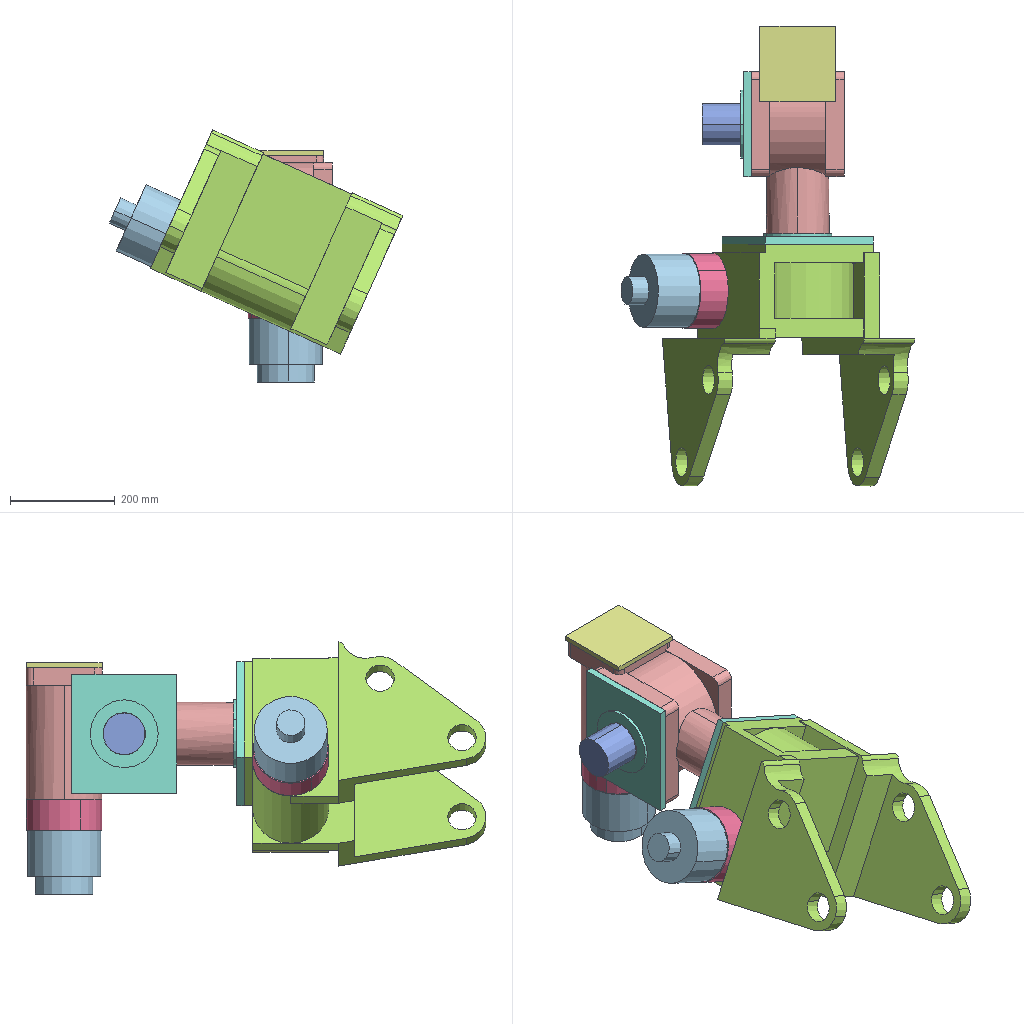Assembly | SolidWorks | 9 different items | 22 placed | box 561 x 878 x 481 mm
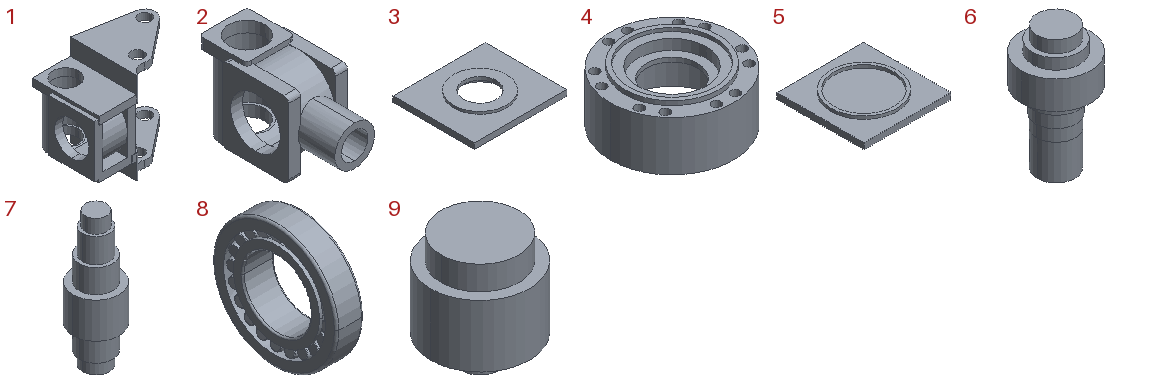Parts list (item | quantity | size | volume | features):
1 | x1 | 461.6 x 289.885 x 398 mm | 8973124 mm3 | features ICE 16, Extrusion 1, MirrorPattern 1
2 | x1 | 178 x 397.308 x 252 mm | 4609278 mm3 | features ICE 12, Extrusion 1, Fillet 1
3 | x2 | 227 x 200 x 28 mm | 588836 mm3 | features ICE 4, Extrusion 1
4 | x2 | 144 x 144 x 63 mm | 426591 mm3 | features ICE 5, Extrusion 1, HoleWzd 1
5 | x2 | 145 x 145 x 15 mm | 218497 mm3 | features Extrusion 1, ICE 1
6 | x2 | 145.723 x 145.723 x 263.5 mm | 2176439 mm3 | features ICE 6, Extrusion 1
7 | x2 | 103.893 x 103.893 x 300 mm | 1437259 mm3 | features ICE 5, Extrusion 1
8 | x8 | 29.75 x 110 x 110 mm | 137070 mm3 | features Revolution 3, CirPattern 1
9 | x2 | 140 x 140 x 156 mm | 1755635 mm3 | features ICE 2, Extrusion 1
Mates (type | each side: item.copy, entity, surface, feature):
Concentric | 2.1 face cylinder Boss-Extrude6 | 6.1 face cylinder Boss-Extrude7
Coincident | 2.1 face plane Boss-Extrude7 | 6.1 face plane Boss-Extrude7
Coincident | 6.1 face plane Boss-Extrude1 | 1.1 face plane Cut-Extrude5
Concentric | 6.1 face cylinder Boss-Extrude3 | 1.1 face cylinder Cut-Extrude4
Coincident | 2.1 face plane Cut-Extrude5 | 6.2 face plane Boss-Extrude1
Concentric | 2.1 face cylinder Cut-Extrude4 | 6.2 face cylinder Boss-Extrude3
Concentric | 1.1 face cylinder Cut-Extrude3 | 7.1 face cylinder Boss-Extrude3
DistanceDim | 7.1 face plane Boss-Extrude1 | 1.1 face plane Boss-Extrude1
Concentric | 2.1 face cylinder Cut-Extrude2 | 7.2 face cylinder Boss-Extrude3
DistanceDim | 7.2 face plane Boss-Extrude1 | 2.1 face plane Boss-Extrude1
Concentric | 6.1 face cylinder Boss-Extrude1 | 8.1 face cylinder Revolve1
Coincident | 6.1 face plane Boss-Extrude2 | 8.1 face plane Revolve1
Concentric | 6.1 face cylinder Boss-Extrude5 | 8.2 face cylinder Revolve1
Coincident | 6.1 face plane Boss-Extrude4 | 8.2 face plane Revolve1
Coincident | 3.1 face plane Boss-Extrude1 | 1.1 face plane Boss-Extrude5
Concentric | 6.1 face cylinder Boss-Extrude7 | 3.1 face cylinder Cut-Extrude1
Coincident | 1.1 face plane Boss-Extrude5 | 3.1 face plane Boss-Extrude1
Concentric | 6.2 face cylinder Boss-Extrude7 | 8.3 face cylinder Revolve1
Coincident | 6.2 face plane Boss-Extrude4 | 8.3 face plane Revolve1
Coincident | 2.1 face plane Boss-Extrude5 | 3.2 face plane Boss-Extrude1 | 2 times
Concentric | 6.2 face cylinder Boss-Extrude7 | 3.2 face cylinder Cut-Extrude1
Coincident | 6.2 face plane Boss-Extrude2 | 8.4 face plane Revolve1
Concentric | 6.2 face cylinder Boss-Extrude1 | 8.4 face cylinder Revolve1
Coincident | 7.2 face plane Boss-Extrude4 | 8.5 face plane Revolve1
Concentric | 7.2 face cylinder Boss-Extrude6 | 8.5 face cylinder Revolve1
Coincident | 7.2 face plane Boss-Extrude2 | 8.6 face plane Revolve1
Concentric | 7.2 face cylinder Boss-Extrude1 | 8.6 face cylinder Revolve1
Coincident | 7.1 face plane Boss-Extrude2 | 8.7 face plane Revolve1
Concentric | 7.1 face cylinder Boss-Extrude1 | 8.8 face cylinder Revolve1
Concentric | 7.1 face cylinder Boss-Extrude1 | 8.7 face cylinder Revolve1
Coincident | 7.1 face plane Boss-Extrude4 | 8.8 face plane Revolve1
Concentric | 7.2 face cylinder Boss-Extrude6 | 4.1 face cylinder Boss-Extrude1
Coincident | 2.1 face plane Boss-Extrude1 | 4.1 face plane Boss-Extrude1
Coincident | 4.1 face plane Boss-Extrude1 | 9.1 face plane Boss-Extrude2
Concentric | 4.1 face cylinder Boss-Extrude1 | 9.1 face cylinder Boss-Extrude2
Coincident | 1.1 face plane Boss-Extrude1 | 4.2 face plane Boss-Extrude1
Concentric | 7.1 face cylinder Boss-Extrude6 | 4.2 face cylinder Cut-Extrude1
Coincident | 9.2 face plane Boss-Extrude2 | 4.2 face plane Boss-Extrude1
Concentric | 9.2 face cylinder Boss-Extrude2 | 4.2 face cylinder Boss-Extrude1
Concentric | 2.1 face cylinder Cut-Extrude2 | 5.1 face cylinder Boss-Extrude2
Coincident | 2.1 face plane Boss-Extrude1 | 5.1 face plane Boss-Extrude1
Coincident | 2.1 face plane Boss-Extrude2 | 5.1 face plane Boss-Extrude1
Concentric | 1.1 face cylinder Cut-Extrude2 | 5.2 face cylinder Boss-Extrude2
Coincident | 1.1 face plane Boss-Extrude1 | 5.2 face plane Boss-Extrude1
Coincident | 1.1 face plane Boss-Extrude2 | 5.2 face plane Boss-Extrude1